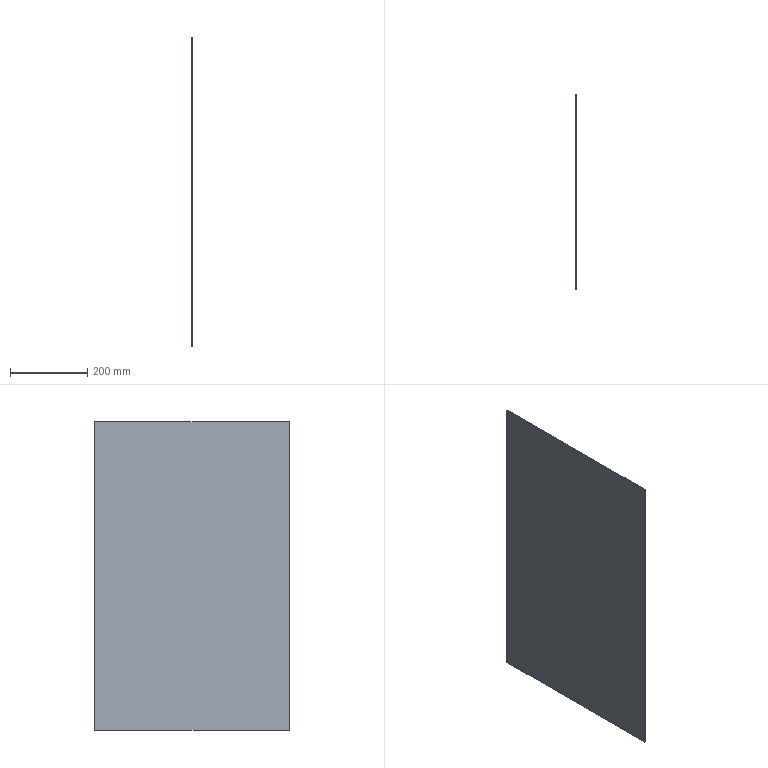Part | SolidWorks | 1 solid | 6 faces | box 1.5 x 505 x 800 mm | volume 606000 mm3 | plane 6
STEP:
#1=CARTESIAN_POINT('',(0.,252.5,400.));
#2=VERTEX_POINT('',#1);
#3=CARTESIAN_POINT('',(0.,-252.5,400.));
#4=VERTEX_POINT('',#3);
#5=CARTESIAN_POINT('',(0.,-252.5,400.));
#6=DIRECTION('',(0.,-1.,0.));
#7=VECTOR('',#6,1000.);
#8=LINE('',#5,#7);
#9=EDGE_CURVE('',#2,#4,#8,.T.);
#10=ORIENTED_EDGE('',*,*,#9,.F.);
#11=CARTESIAN_POINT('',(-1.5,252.5,400.));
#12=VERTEX_POINT('',#11);
#13=CARTESIAN_POINT('',(-1.5,252.5,400.));
#14=DIRECTION('',(1.,0.,0.));
#15=VECTOR('',#14,1000.);
#16=LINE('',#13,#15);
#17=EDGE_CURVE('',#12,#2,#16,.T.);
#18=ORIENTED_EDGE('',*,*,#17,.F.);
#19=CARTESIAN_POINT('',(-1.5,-252.5,400.));
#20=VERTEX_POINT('',#19);
#21=CARTESIAN_POINT('',(-1.5,-252.5,400.));
#22=DIRECTION('',(0.,-1.,0.));
#23=VECTOR('',#22,1000.);
#24=LINE('',#21,#23);
#25=EDGE_CURVE('',#12,#20,#24,.T.);
#26=ORIENTED_EDGE('',*,*,#25,.T.);
#27=CARTESIAN_POINT('',(-1.5,-252.5,400.));
#28=DIRECTION('',(1.,0.,0.));
#29=VECTOR('',#28,1000.);
#30=LINE('',#27,#29);
#31=EDGE_CURVE('',#20,#4,#30,.T.);
#32=ORIENTED_EDGE('',*,*,#31,.T.);
#33=EDGE_LOOP('',(#10,#18,#26,#32));
#34=FACE_OUTER_BOUND('',#33,.T.);
#35=CARTESIAN_POINT('',(-1.5,-252.5,400.));
#36=DIRECTION('',(0.,0.,1.));
#37=DIRECTION('',(1.,0.,0.));
#38=AXIS2_PLACEMENT_3D('',#35,#36,#37);
#39=PLANE('',#38);
#40=ADVANCED_FACE('',(#34),#39,.T.);
#41=CARTESIAN_POINT('',(0.,252.5,-400.));
#42=VERTEX_POINT('',#41);
#43=CARTESIAN_POINT('',(0.,252.5,-400.));
#44=DIRECTION('',(0.,0.,1.));
#45=VECTOR('',#44,1000.);
#46=LINE('',#43,#45);
#47=EDGE_CURVE('',#42,#2,#46,.T.);
#48=ORIENTED_EDGE('',*,*,#47,.F.);
#49=CARTESIAN_POINT('',(-1.5,252.5,-400.));
#50=VERTEX_POINT('',#49);
#51=CARTESIAN_POINT('',(-1.5,252.5,-400.));
#52=DIRECTION('',(1.,0.,0.));
#53=VECTOR('',#52,1000.);
#54=LINE('',#51,#53);
#55=EDGE_CURVE('',#50,#42,#54,.T.);
#56=ORIENTED_EDGE('',*,*,#55,.F.);
#57=CARTESIAN_POINT('',(-1.5,252.5,-400.));
#58=DIRECTION('',(0.,0.,1.));
#59=VECTOR('',#58,1000.);
#60=LINE('',#57,#59);
#61=EDGE_CURVE('',#50,#12,#60,.T.);
#62=ORIENTED_EDGE('',*,*,#61,.T.);
#63=ORIENTED_EDGE('',*,*,#17,.T.);
#64=EDGE_LOOP('',(#48,#56,#62,#63));
#65=FACE_OUTER_BOUND('',#64,.T.);
#66=CARTESIAN_POINT('',(-1.5,252.5,-400.));
#67=DIRECTION('',(0.,1.,0.));
#68=DIRECTION('',(0.,0.,1.));
#69=AXIS2_PLACEMENT_3D('',#66,#67,#68);
#70=PLANE('',#69);
#71=ADVANCED_FACE('',(#65),#70,.T.);
#72=CARTESIAN_POINT('',(0.,-252.5,-400.));
#73=VERTEX_POINT('',#72);
#74=CARTESIAN_POINT('',(0.,-252.5,-400.));
#75=DIRECTION('',(0.,1.,0.));
#76=VECTOR('',#75,1000.);
#77=LINE('',#74,#76);
#78=EDGE_CURVE('',#73,#42,#77,.T.);
#79=ORIENTED_EDGE('',*,*,#78,.F.);
#80=CARTESIAN_POINT('',(-1.5,-252.5,-400.));
#81=VERTEX_POINT('',#80);
#82=CARTESIAN_POINT('',(-1.5,-252.5,-400.));
#83=DIRECTION('',(1.,0.,0.));
#84=VECTOR('',#83,1000.);
#85=LINE('',#82,#84);
#86=EDGE_CURVE('',#81,#73,#85,.T.);
#87=ORIENTED_EDGE('',*,*,#86,.F.);
#88=CARTESIAN_POINT('',(-1.5,-252.5,-400.));
#89=DIRECTION('',(0.,1.,0.));
#90=VECTOR('',#89,1000.);
#91=LINE('',#88,#90);
#92=EDGE_CURVE('',#81,#50,#91,.T.);
#93=ORIENTED_EDGE('',*,*,#92,.T.);
#94=ORIENTED_EDGE('',*,*,#55,.T.);
#95=EDGE_LOOP('',(#79,#87,#93,#94));
#96=FACE_OUTER_BOUND('',#95,.T.);
#97=CARTESIAN_POINT('',(-1.5,-252.5,-400.));
#98=DIRECTION('',(0.,0.,-1.));
#99=DIRECTION('',(-1.,0.,0.));
#100=AXIS2_PLACEMENT_3D('',#97,#98,#99);
#101=PLANE('',#100);
#102=ADVANCED_FACE('',(#96),#101,.T.);
#103=CARTESIAN_POINT('',(0.,-252.5,-400.));
#104=DIRECTION('',(0.,0.,-1.));
#105=VECTOR('',#104,1000.);
#106=LINE('',#103,#105);
#107=EDGE_CURVE('',#4,#73,#106,.T.);
#108=ORIENTED_EDGE('',*,*,#107,.F.);
#109=ORIENTED_EDGE('',*,*,#31,.F.);
#110=CARTESIAN_POINT('',(-1.5,-252.5,-400.));
#111=DIRECTION('',(0.,0.,-1.));
#112=VECTOR('',#111,1000.);
#113=LINE('',#110,#112);
#114=EDGE_CURVE('',#20,#81,#113,.T.);
#115=ORIENTED_EDGE('',*,*,#114,.T.);
#116=ORIENTED_EDGE('',*,*,#86,.T.);
#117=EDGE_LOOP('',(#108,#109,#115,#116));
#118=FACE_OUTER_BOUND('',#117,.T.);
#119=CARTESIAN_POINT('',(-1.5,-252.5,-400.));
#120=DIRECTION('',(0.,-1.,0.));
#121=DIRECTION('',(0.,0.,-1.));
#122=AXIS2_PLACEMENT_3D('',#119,#120,#121);
#123=PLANE('',#122);
#124=ADVANCED_FACE('',(#118),#123,.T.);
#125=ORIENTED_EDGE('',*,*,#25,.F.);
#126=ORIENTED_EDGE('',*,*,#61,.F.);
#127=ORIENTED_EDGE('',*,*,#92,.F.);
#128=ORIENTED_EDGE('',*,*,#114,.F.);
#129=EDGE_LOOP('',(#125,#126,#127,#128));
#130=FACE_OUTER_BOUND('',#129,.T.);
#131=CARTESIAN_POINT('',(-1.5,0.,0.));
#132=DIRECTION('',(1.,0.,0.));
#133=DIRECTION('',(0.,0.,-1.));
#134=AXIS2_PLACEMENT_3D('',#131,#132,#133);
#135=PLANE('',#134);
#136=ADVANCED_FACE('',(#130),#135,.F.);
#137=ORIENTED_EDGE('',*,*,#9,.T.);
#138=ORIENTED_EDGE('',*,*,#107,.T.);
#139=ORIENTED_EDGE('',*,*,#78,.T.);
#140=ORIENTED_EDGE('',*,*,#47,.T.);
#141=EDGE_LOOP('',(#137,#138,#139,#140));
#142=FACE_OUTER_BOUND('',#141,.T.);
#143=CARTESIAN_POINT('',(0.,0.,0.));
#144=DIRECTION('',(1.,0.,0.));
#145=DIRECTION('',(0.,0.,-1.));
#146=AXIS2_PLACEMENT_3D('',#143,#144,#145);
#147=PLANE('',#146);
#148=ADVANCED_FACE('',(#142),#147,.T.);
#149=CLOSED_SHELL('',(#40,#71,#102,#124,#136,#148));
#150=MANIFOLD_SOLID_BREP('',#149);
#151=CARTESIAN_POINT('',(0.,0.,0.));
#152=DIRECTION('',(0.,0.,1.));
#153=DIRECTION('',(1.,0.,0.));
#154=AXIS2_PLACEMENT_3D('',#151,#152,#153);
#155=(LENGTH_UNIT()NAMED_UNIT(*)SI_UNIT(.MILLI.,.METRE.));
#156=UNCERTAINTY_MEASURE_WITH_UNIT(LENGTH_MEASURE(0.00001),#155,'','');
#157=(NAMED_UNIT(*)PLANE_ANGLE_UNIT()SI_UNIT($,.RADIAN.));
#158=(NAMED_UNIT(*)SI_UNIT($,.STERADIAN.)SOLID_ANGLE_UNIT());
#159=(GEOMETRIC_REPRESENTATION_CONTEXT(3)GLOBAL_UNCERTAINTY_ASSIGNED_CONTEXT((#156))GLOBAL_UNIT_ASSIGNED_CONTEXT((#155,#157,#158))REPRESENTATION_CONTEXT('',''));
#160=ADVANCED_BREP_SHAPE_REPRESENTATION('',(#150,#154),#159);